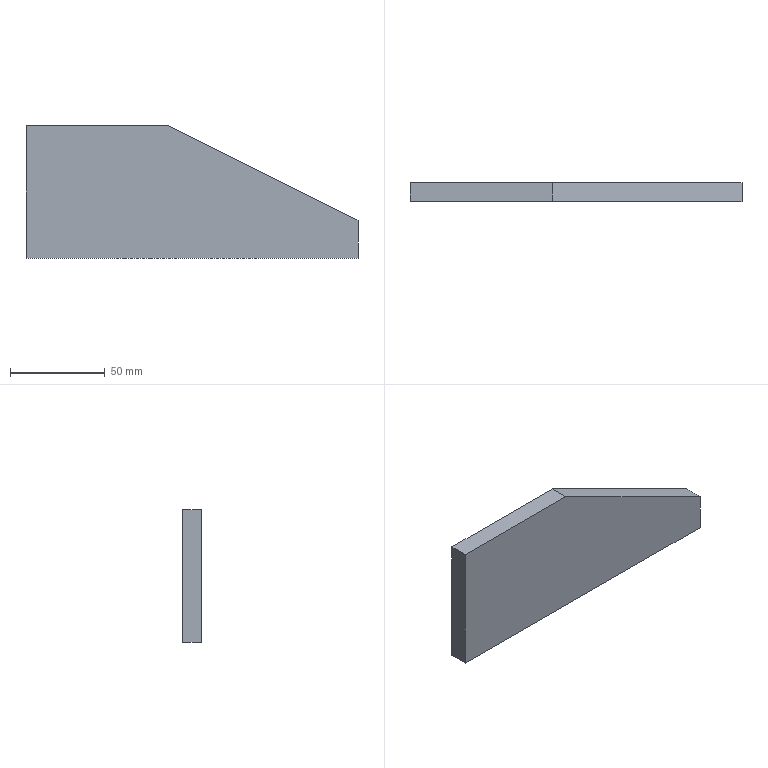Part | STEP file | Positioning_id2130_x_t | 1 solid | 7 faces | box 175 x 10 x 70 mm | volume 97500 mm3 | plane 7
STEP:
#1=CARTESIAN_POINT('',(0.,0.,0.));
#2=DIRECTION('',(0.,0.,1.));
#3=DIRECTION('',(1.,0.,0.));
#4=AXIS2_PLACEMENT_3D('',#1,#2,#3);
#5=CARTESIAN_POINT('',(-823.002,196.5,393.532));
#6=VERTEX_POINT('',#5);
#7=CARTESIAN_POINT('',(-923.002,196.5,443.532));
#8=VERTEX_POINT('',#7);
#9=CARTESIAN_POINT('',(-823.002,196.5,393.532));
#10=DIRECTION('',(-0.8944,0.,0.4472));
#11=VECTOR('',#10,1.);
#12=LINE('',#9,#11);
#13=CARTESIAN_POINT('',(-923.002,201.5,443.532));
#14=DIRECTION('',(-0.4472,0.,-0.8944));
#15=DIRECTION('',(0.8944,0.,-0.4472));
#16=AXIS2_PLACEMENT_3D('',#13,#14,#15);
#17=PLANE('',#16);
#18=CARTESIAN_POINT('',(111.803,5.));
#19=DIRECTION('',(-1.,0.));
#20=VECTOR('',#19,1.);
#21=LINE('',#18,#20);
#22=(GEOMETRIC_REPRESENTATION_CONTEXT(2)PARAMETRIC_REPRESENTATION_CONTEXT()REPRESENTATION_CONTEXT('',''));
#23=DEFINITIONAL_REPRESENTATION('',(#21),#22);
#24=PCURVE('',#17,#23);
#25=CARTESIAN_POINT('',(-893.002,196.5,413.532));
#26=DIRECTION('',(0.,-1.,0.));
#27=DIRECTION('',(1.,0.,0.));
#28=AXIS2_PLACEMENT_3D('',#25,#26,#27);
#29=PLANE('',#28);
#30=CARTESIAN_POINT('',(70.,-20.));
#31=DIRECTION('',(-0.8944,0.4472));
#32=VECTOR('',#31,1.);
#33=LINE('',#30,#32);
#34=(GEOMETRIC_REPRESENTATION_CONTEXT(2)PARAMETRIC_REPRESENTATION_CONTEXT()REPRESENTATION_CONTEXT('',''));
#35=DEFINITIONAL_REPRESENTATION('',(#33),#34);
#36=PCURVE('',#29,#35);
#37=SURFACE_CURVE('',#12,(#24,#36),.PCURVE_S1.);
#38=EDGE_CURVE('',#6,#8,#37,.T.);
#39=ORIENTED_EDGE('',*,*,#38,.F.);
#40=CARTESIAN_POINT('',(-823.002,206.5,393.532));
#41=VERTEX_POINT('',#40);
#42=CARTESIAN_POINT('',(-823.002,206.5,393.532));
#43=DIRECTION('',(0.,-1.,0.));
#44=VECTOR('',#43,1.);
#45=LINE('',#42,#44);
#46=CARTESIAN_POINT('',(111.803,-5.));
#47=DIRECTION('',(0.,1.));
#48=VECTOR('',#47,1.);
#49=LINE('',#46,#48);
#50=(GEOMETRIC_REPRESENTATION_CONTEXT(2)PARAMETRIC_REPRESENTATION_CONTEXT()REPRESENTATION_CONTEXT('',''));
#51=DEFINITIONAL_REPRESENTATION('',(#49),#50);
#52=PCURVE('',#17,#51);
#53=CARTESIAN_POINT('',(-823.002,201.5,413.532));
#54=DIRECTION('',(1.,0.,0.));
#55=DIRECTION('',(0.,1.,0.));
#56=AXIS2_PLACEMENT_3D('',#53,#54,#55);
#57=PLANE('',#56);
#58=CARTESIAN_POINT('',(5.,-20.));
#59=DIRECTION('',(-1.,0.));
#60=VECTOR('',#59,1.);
#61=LINE('',#58,#60);
#62=(GEOMETRIC_REPRESENTATION_CONTEXT(2)PARAMETRIC_REPRESENTATION_CONTEXT()REPRESENTATION_CONTEXT('',''));
#63=DEFINITIONAL_REPRESENTATION('',(#61),#62);
#64=PCURVE('',#57,#63);
#65=SURFACE_CURVE('',#45,(#52,#64),.PCURVE_S1.);
#66=EDGE_CURVE('',#41,#6,#65,.T.);
#67=ORIENTED_EDGE('',*,*,#66,.F.);
#68=CARTESIAN_POINT('',(-923.002,206.5,443.532));
#69=VERTEX_POINT('',#68);
#70=CARTESIAN_POINT('',(-923.002,206.5,443.532));
#71=DIRECTION('',(0.8944,0.,-0.4472));
#72=VECTOR('',#71,1.);
#73=LINE('',#70,#72);
#74=CARTESIAN_POINT('',(0.,-5.));
#75=DIRECTION('',(1.,0.));
#76=VECTOR('',#75,1.);
#77=LINE('',#74,#76);
#78=(GEOMETRIC_REPRESENTATION_CONTEXT(2)PARAMETRIC_REPRESENTATION_CONTEXT()REPRESENTATION_CONTEXT('',''));
#79=DEFINITIONAL_REPRESENTATION('',(#77),#78);
#80=PCURVE('',#17,#79);
#81=CARTESIAN_POINT('',(-893.002,206.5,413.532));
#82=DIRECTION('',(0.,1.,0.));
#83=DIRECTION('',(-1.,0.,0.));
#84=AXIS2_PLACEMENT_3D('',#81,#82,#83);
#85=PLANE('',#84);
#86=CARTESIAN_POINT('',(30.,30.));
#87=DIRECTION('',(-0.8944,-0.4472));
#88=VECTOR('',#87,1.);
#89=LINE('',#86,#88);
#90=(GEOMETRIC_REPRESENTATION_CONTEXT(2)PARAMETRIC_REPRESENTATION_CONTEXT()REPRESENTATION_CONTEXT('',''));
#91=DEFINITIONAL_REPRESENTATION('',(#89),#90);
#92=PCURVE('',#85,#91);
#93=SURFACE_CURVE('',#73,(#80,#92),.PCURVE_S1.);
#94=EDGE_CURVE('',#69,#41,#93,.T.);
#95=ORIENTED_EDGE('',*,*,#94,.F.);
#96=CARTESIAN_POINT('',(-923.002,196.5,443.532));
#97=DIRECTION('',(0.,1.,0.));
#98=VECTOR('',#97,1.);
#99=LINE('',#96,#98);
#100=CARTESIAN_POINT('',(0.,5.));
#101=DIRECTION('',(0.,-1.));
#102=VECTOR('',#101,1.);
#103=LINE('',#100,#102);
#104=(GEOMETRIC_REPRESENTATION_CONTEXT(2)PARAMETRIC_REPRESENTATION_CONTEXT()REPRESENTATION_CONTEXT('',''));
#105=DEFINITIONAL_REPRESENTATION('',(#103),#104);
#106=PCURVE('',#17,#105);
#107=CARTESIAN_POINT('',(-893.002,201.5,443.532));
#108=DIRECTION('',(0.,0.,1.));
#109=DIRECTION('',(0.,-1.,0.));
#110=AXIS2_PLACEMENT_3D('',#107,#108,#109);
#111=PLANE('',#110);
#112=CARTESIAN_POINT('',(5.,-30.));
#113=DIRECTION('',(-1.,0.));
#114=VECTOR('',#113,1.);
#115=LINE('',#112,#114);
#116=(GEOMETRIC_REPRESENTATION_CONTEXT(2)PARAMETRIC_REPRESENTATION_CONTEXT()REPRESENTATION_CONTEXT('',''));
#117=DEFINITIONAL_REPRESENTATION('',(#115),#116);
#118=PCURVE('',#111,#117);
#119=SURFACE_CURVE('',#99,(#106,#118),.PCURVE_S1.);
#120=EDGE_CURVE('',#8,#69,#119,.T.);
#121=ORIENTED_EDGE('',*,*,#120,.F.);
#122=EDGE_LOOP('',(#39,#67,#95,#121));
#123=FACE_BOUND('',#122,.T.);
#124=ADVANCED_FACE('',(#123),#17,.F.);
#125=CARTESIAN_POINT('',(-823.002,206.5,373.532));
#126=VERTEX_POINT('',#125);
#127=CARTESIAN_POINT('',(-823.002,206.5,393.532));
#128=DIRECTION('',(0.,0.,-1.));
#129=VECTOR('',#128,1.);
#130=LINE('',#127,#129);
#131=CARTESIAN_POINT('',(5.,-20.));
#132=DIRECTION('',(0.,-1.));
#133=VECTOR('',#132,1.);
#134=LINE('',#131,#133);
#135=(GEOMETRIC_REPRESENTATION_CONTEXT(2)PARAMETRIC_REPRESENTATION_CONTEXT()REPRESENTATION_CONTEXT('',''));
#136=DEFINITIONAL_REPRESENTATION('',(#134),#135);
#137=PCURVE('',#57,#136);
#138=CARTESIAN_POINT('',(-70.,-20.));
#139=DIRECTION('',(0.,-1.));
#140=VECTOR('',#139,1.);
#141=LINE('',#138,#140);
#142=(GEOMETRIC_REPRESENTATION_CONTEXT(2)PARAMETRIC_REPRESENTATION_CONTEXT()REPRESENTATION_CONTEXT('',''));
#143=DEFINITIONAL_REPRESENTATION('',(#141),#142);
#144=PCURVE('',#85,#143);
#145=SURFACE_CURVE('',#130,(#137,#144),.PCURVE_S1.);
#146=EDGE_CURVE('',#41,#126,#145,.T.);
#147=ORIENTED_EDGE('',*,*,#146,.F.);
#148=ORIENTED_EDGE('',*,*,#66,.T.);
#149=CARTESIAN_POINT('',(-823.002,196.5,373.532));
#150=VERTEX_POINT('',#149);
#151=CARTESIAN_POINT('',(-823.002,196.5,373.532));
#152=DIRECTION('',(0.,0.,1.));
#153=VECTOR('',#152,1.);
#154=LINE('',#151,#153);
#155=CARTESIAN_POINT('',(-5.,-40.));
#156=DIRECTION('',(0.,1.));
#157=VECTOR('',#156,1.);
#158=LINE('',#155,#157);
#159=(GEOMETRIC_REPRESENTATION_CONTEXT(2)PARAMETRIC_REPRESENTATION_CONTEXT()REPRESENTATION_CONTEXT('',''));
#160=DEFINITIONAL_REPRESENTATION('',(#158),#159);
#161=PCURVE('',#57,#160);
#162=CARTESIAN_POINT('',(70.,-40.));
#163=DIRECTION('',(0.,1.));
#164=VECTOR('',#163,1.);
#165=LINE('',#162,#164);
#166=(GEOMETRIC_REPRESENTATION_CONTEXT(2)PARAMETRIC_REPRESENTATION_CONTEXT()REPRESENTATION_CONTEXT('',''));
#167=DEFINITIONAL_REPRESENTATION('',(#165),#166);
#168=PCURVE('',#29,#167);
#169=SURFACE_CURVE('',#154,(#161,#168),.PCURVE_S1.);
#170=EDGE_CURVE('',#150,#6,#169,.T.);
#171=ORIENTED_EDGE('',*,*,#170,.F.);
#172=CARTESIAN_POINT('',(-823.002,196.5,373.532));
#173=DIRECTION('',(0.,1.,0.));
#174=VECTOR('',#173,1.);
#175=LINE('',#172,#174);
#176=CARTESIAN_POINT('',(-5.,-40.));
#177=DIRECTION('',(1.,0.));
#178=VECTOR('',#177,1.);
#179=LINE('',#176,#178);
#180=(GEOMETRIC_REPRESENTATION_CONTEXT(2)PARAMETRIC_REPRESENTATION_CONTEXT()REPRESENTATION_CONTEXT('',''));
#181=DEFINITIONAL_REPRESENTATION('',(#179),#180);
#182=PCURVE('',#57,#181);
#183=CARTESIAN_POINT('',(-893.002,201.5,373.532));
#184=DIRECTION('',(0.,0.,-1.));
#185=DIRECTION('',(0.,1.,0.));
#186=AXIS2_PLACEMENT_3D('',#183,#184,#185);
#187=PLANE('',#186);
#188=CARTESIAN_POINT('',(-5.,70.));
#189=DIRECTION('',(1.,0.));
#190=VECTOR('',#189,1.);
#191=LINE('',#188,#190);
#192=(GEOMETRIC_REPRESENTATION_CONTEXT(2)PARAMETRIC_REPRESENTATION_CONTEXT()REPRESENTATION_CONTEXT('',''));
#193=DEFINITIONAL_REPRESENTATION('',(#191),#192);
#194=PCURVE('',#187,#193);
#195=SURFACE_CURVE('',#175,(#182,#194),.PCURVE_S1.);
#196=EDGE_CURVE('',#150,#126,#195,.T.);
#197=ORIENTED_EDGE('',*,*,#196,.T.);
#198=EDGE_LOOP('',(#147,#148,#171,#197));
#199=FACE_BOUND('',#198,.T.);
#200=ADVANCED_FACE('',(#199),#57,.T.);
#201=ORIENTED_EDGE('',*,*,#170,.T.);
#202=ORIENTED_EDGE('',*,*,#38,.T.);
#203=CARTESIAN_POINT('',(-998.002,196.5,443.532));
#204=VERTEX_POINT('',#203);
#205=CARTESIAN_POINT('',(-923.002,196.5,443.532));
#206=DIRECTION('',(-1.,0.,0.));
#207=VECTOR('',#206,1.);
#208=LINE('',#205,#207);
#209=CARTESIAN_POINT('',(-30.,30.));
#210=DIRECTION('',(-1.,0.));
#211=VECTOR('',#210,1.);
#212=LINE('',#209,#211);
#213=(GEOMETRIC_REPRESENTATION_CONTEXT(2)PARAMETRIC_REPRESENTATION_CONTEXT()REPRESENTATION_CONTEXT('',''));
#214=DEFINITIONAL_REPRESENTATION('',(#212),#213);
#215=PCURVE('',#29,#214);
#216=CARTESIAN_POINT('',(5.,-30.));
#217=DIRECTION('',(0.,-1.));
#218=VECTOR('',#217,1.);
#219=LINE('',#216,#218);
#220=(GEOMETRIC_REPRESENTATION_CONTEXT(2)PARAMETRIC_REPRESENTATION_CONTEXT()REPRESENTATION_CONTEXT('',''));
#221=DEFINITIONAL_REPRESENTATION('',(#219),#220);
#222=PCURVE('',#111,#221);
#223=SURFACE_CURVE('',#208,(#215,#222),.PCURVE_S1.);
#224=EDGE_CURVE('',#8,#204,#223,.T.);
#225=ORIENTED_EDGE('',*,*,#224,.T.);
#226=CARTESIAN_POINT('',(-998.002,196.5,373.532));
#227=VERTEX_POINT('',#226);
#228=CARTESIAN_POINT('',(-998.002,196.5,443.532));
#229=DIRECTION('',(0.,0.,-1.));
#230=VECTOR('',#229,1.);
#231=LINE('',#228,#230);
#232=CARTESIAN_POINT('',(-105.,30.));
#233=DIRECTION('',(0.,-1.));
#234=VECTOR('',#233,1.);
#235=LINE('',#232,#234);
#236=(GEOMETRIC_REPRESENTATION_CONTEXT(2)PARAMETRIC_REPRESENTATION_CONTEXT()REPRESENTATION_CONTEXT('',''));
#237=DEFINITIONAL_REPRESENTATION('',(#235),#236);
#238=PCURVE('',#29,#237);
#239=CARTESIAN_POINT('',(-998.002,201.5,413.532));
#240=DIRECTION('',(-1.,0.,0.));
#241=DIRECTION('',(0.,-1.,0.));
#242=AXIS2_PLACEMENT_3D('',#239,#240,#241);
#243=PLANE('',#242);
#244=CARTESIAN_POINT('',(5.,30.));
#245=DIRECTION('',(0.,-1.));
#246=VECTOR('',#245,1.);
#247=LINE('',#244,#246);
#248=(GEOMETRIC_REPRESENTATION_CONTEXT(2)PARAMETRIC_REPRESENTATION_CONTEXT()REPRESENTATION_CONTEXT('',''));
#249=DEFINITIONAL_REPRESENTATION('',(#247),#248);
#250=PCURVE('',#243,#249);
#251=SURFACE_CURVE('',#231,(#238,#250),.PCURVE_S1.);
#252=EDGE_CURVE('',#204,#227,#251,.T.);
#253=ORIENTED_EDGE('',*,*,#252,.T.);
#254=CARTESIAN_POINT('',(-998.002,196.5,373.532));
#255=DIRECTION('',(1.,0.,0.));
#256=VECTOR('',#255,1.);
#257=LINE('',#254,#256);
#258=CARTESIAN_POINT('',(-105.,-40.));
#259=DIRECTION('',(1.,0.));
#260=VECTOR('',#259,1.);
#261=LINE('',#258,#260);
#262=(GEOMETRIC_REPRESENTATION_CONTEXT(2)PARAMETRIC_REPRESENTATION_CONTEXT()REPRESENTATION_CONTEXT('',''));
#263=DEFINITIONAL_REPRESENTATION('',(#261),#262);
#264=PCURVE('',#29,#263);
#265=CARTESIAN_POINT('',(-5.,-105.));
#266=DIRECTION('',(0.,1.));
#267=VECTOR('',#266,1.);
#268=LINE('',#265,#267);
#269=(GEOMETRIC_REPRESENTATION_CONTEXT(2)PARAMETRIC_REPRESENTATION_CONTEXT()REPRESENTATION_CONTEXT('',''));
#270=DEFINITIONAL_REPRESENTATION('',(#268),#269);
#271=PCURVE('',#187,#270);
#272=SURFACE_CURVE('',#257,(#264,#271),.PCURVE_S1.);
#273=EDGE_CURVE('',#227,#150,#272,.T.);
#274=ORIENTED_EDGE('',*,*,#273,.T.);
#275=EDGE_LOOP('',(#201,#202,#225,#253,#274));
#276=FACE_BOUND('',#275,.T.);
#277=ADVANCED_FACE('',(#276),#29,.T.);
#278=ORIENTED_EDGE('',*,*,#224,.F.);
#279=ORIENTED_EDGE('',*,*,#120,.T.);
#280=CARTESIAN_POINT('',(-998.002,206.5,443.532));
#281=VERTEX_POINT('',#280);
#282=CARTESIAN_POINT('',(-998.002,206.5,443.532));
#283=DIRECTION('',(1.,0.,0.));
#284=VECTOR('',#283,1.);
#285=LINE('',#282,#284);
#286=CARTESIAN_POINT('',(-5.,-105.));
#287=DIRECTION('',(0.,1.));
#288=VECTOR('',#287,1.);
#289=LINE('',#286,#288);
#290=(GEOMETRIC_REPRESENTATION_CONTEXT(2)PARAMETRIC_REPRESENTATION_CONTEXT()REPRESENTATION_CONTEXT('',''));
#291=DEFINITIONAL_REPRESENTATION('',(#289),#290);
#292=PCURVE('',#111,#291);
#293=CARTESIAN_POINT('',(105.,30.));
#294=DIRECTION('',(-1.,0.));
#295=VECTOR('',#294,1.);
#296=LINE('',#293,#295);
#297=(GEOMETRIC_REPRESENTATION_CONTEXT(2)PARAMETRIC_REPRESENTATION_CONTEXT()REPRESENTATION_CONTEXT('',''));
#298=DEFINITIONAL_REPRESENTATION('',(#296),#297);
#299=PCURVE('',#85,#298);
#300=SURFACE_CURVE('',#285,(#292,#299),.PCURVE_S1.);
#301=EDGE_CURVE('',#281,#69,#300,.T.);
#302=ORIENTED_EDGE('',*,*,#301,.F.);
#303=CARTESIAN_POINT('',(-998.002,196.5,443.532));
#304=DIRECTION('',(0.,1.,0.));
#305=VECTOR('',#304,1.);
#306=LINE('',#303,#305);
#307=CARTESIAN_POINT('',(5.,-105.));
#308=DIRECTION('',(-1.,0.));
#309=VECTOR('',#308,1.);
#310=LINE('',#307,#309);
#311=(GEOMETRIC_REPRESENTATION_CONTEXT(2)PARAMETRIC_REPRESENTATION_CONTEXT()REPRESENTATION_CONTEXT('',''));
#312=DEFINITIONAL_REPRESENTATION('',(#310),#311);
#313=PCURVE('',#111,#312);
#314=CARTESIAN_POINT('',(5.,30.));
#315=DIRECTION('',(-1.,0.));
#316=VECTOR('',#315,1.);
#317=LINE('',#314,#316);
#318=(GEOMETRIC_REPRESENTATION_CONTEXT(2)PARAMETRIC_REPRESENTATION_CONTEXT()REPRESENTATION_CONTEXT('',''));
#319=DEFINITIONAL_REPRESENTATION('',(#317),#318);
#320=PCURVE('',#243,#319);
#321=SURFACE_CURVE('',#306,(#313,#320),.PCURVE_S1.);
#322=EDGE_CURVE('',#204,#281,#321,.T.);
#323=ORIENTED_EDGE('',*,*,#322,.F.);
#324=EDGE_LOOP('',(#278,#279,#302,#323));
#325=FACE_BOUND('',#324,.T.);
#326=ADVANCED_FACE('',(#325),#111,.T.);
#327=CARTESIAN_POINT('',(-998.002,206.5,373.532));
#328=VERTEX_POINT('',#327);
#329=CARTESIAN_POINT('',(-998.002,196.5,373.532));
#330=DIRECTION('',(0.,1.,0.));
#331=VECTOR('',#330,1.);
#332=LINE('',#329,#331);
#333=CARTESIAN_POINT('',(5.,-40.));
#334=DIRECTION('',(-1.,0.));
#335=VECTOR('',#334,1.);
#336=LINE('',#333,#335);
#337=(GEOMETRIC_REPRESENTATION_CONTEXT(2)PARAMETRIC_REPRESENTATION_CONTEXT()REPRESENTATION_CONTEXT('',''));
#338=DEFINITIONAL_REPRESENTATION('',(#336),#337);
#339=PCURVE('',#243,#338);
#340=CARTESIAN_POINT('',(-5.,-105.));
#341=DIRECTION('',(1.,0.));
#342=VECTOR('',#341,1.);
#343=LINE('',#340,#342);
#344=(GEOMETRIC_REPRESENTATION_CONTEXT(2)PARAMETRIC_REPRESENTATION_CONTEXT()REPRESENTATION_CONTEXT('',''));
#345=DEFINITIONAL_REPRESENTATION('',(#343),#344);
#346=PCURVE('',#187,#345);
#347=SURFACE_CURVE('',#332,(#339,#346),.PCURVE_S1.);
#348=EDGE_CURVE('',#227,#328,#347,.T.);
#349=ORIENTED_EDGE('',*,*,#348,.F.);
#350=ORIENTED_EDGE('',*,*,#252,.F.);
#351=ORIENTED_EDGE('',*,*,#322,.T.);
#352=CARTESIAN_POINT('',(-998.002,206.5,373.532));
#353=DIRECTION('',(0.,0.,1.));
#354=VECTOR('',#353,1.);
#355=LINE('',#352,#354);
#356=CARTESIAN_POINT('',(-5.,-40.));
#357=DIRECTION('',(0.,1.));
#358=VECTOR('',#357,1.);
#359=LINE('',#356,#358);
#360=(GEOMETRIC_REPRESENTATION_CONTEXT(2)PARAMETRIC_REPRESENTATION_CONTEXT()REPRESENTATION_CONTEXT('',''));
#361=DEFINITIONAL_REPRESENTATION('',(#359),#360);
#362=PCURVE('',#243,#361);
#363=CARTESIAN_POINT('',(105.,-40.));
#364=DIRECTION('',(0.,1.));
#365=VECTOR('',#364,1.);
#366=LINE('',#363,#365);
#367=(GEOMETRIC_REPRESENTATION_CONTEXT(2)PARAMETRIC_REPRESENTATION_CONTEXT()REPRESENTATION_CONTEXT('',''));
#368=DEFINITIONAL_REPRESENTATION('',(#366),#367);
#369=PCURVE('',#85,#368);
#370=SURFACE_CURVE('',#355,(#362,#369),.PCURVE_S1.);
#371=EDGE_CURVE('',#328,#281,#370,.T.);
#372=ORIENTED_EDGE('',*,*,#371,.F.);
#373=EDGE_LOOP('',(#349,#350,#351,#372));
#374=FACE_BOUND('',#373,.T.);
#375=ADVANCED_FACE('',(#374),#243,.T.);
#376=ORIENTED_EDGE('',*,*,#196,.F.);
#377=ORIENTED_EDGE('',*,*,#273,.F.);
#378=ORIENTED_EDGE('',*,*,#348,.T.);
#379=CARTESIAN_POINT('',(-823.002,206.5,373.532));
#380=DIRECTION('',(-1.,0.,0.));
#381=VECTOR('',#380,1.);
#382=LINE('',#379,#381);
#383=CARTESIAN_POINT('',(5.,70.));
#384=DIRECTION('',(0.,-1.));
#385=VECTOR('',#384,1.);
#386=LINE('',#383,#385);
#387=(GEOMETRIC_REPRESENTATION_CONTEXT(2)PARAMETRIC_REPRESENTATION_CONTEXT()REPRESENTATION_CONTEXT('',''));
#388=DEFINITIONAL_REPRESENTATION('',(#386),#387);
#389=PCURVE('',#187,#388);
#390=CARTESIAN_POINT('',(-70.,-40.));
#391=DIRECTION('',(1.,0.));
#392=VECTOR('',#391,1.);
#393=LINE('',#390,#392);
#394=(GEOMETRIC_REPRESENTATION_CONTEXT(2)PARAMETRIC_REPRESENTATION_CONTEXT()REPRESENTATION_CONTEXT('',''));
#395=DEFINITIONAL_REPRESENTATION('',(#393),#394);
#396=PCURVE('',#85,#395);
#397=SURFACE_CURVE('',#382,(#389,#396),.PCURVE_S1.);
#398=EDGE_CURVE('',#126,#328,#397,.T.);
#399=ORIENTED_EDGE('',*,*,#398,.F.);
#400=EDGE_LOOP('',(#376,#377,#378,#399));
#401=FACE_BOUND('',#400,.T.);
#402=ADVANCED_FACE('',(#401),#187,.T.);
#403=ORIENTED_EDGE('',*,*,#301,.T.);
#404=ORIENTED_EDGE('',*,*,#94,.T.);
#405=ORIENTED_EDGE('',*,*,#146,.T.);
#406=ORIENTED_EDGE('',*,*,#398,.T.);
#407=ORIENTED_EDGE('',*,*,#371,.T.);
#408=EDGE_LOOP('',(#403,#404,#405,#406,#407));
#409=FACE_BOUND('',#408,.T.);
#410=ADVANCED_FACE('',(#409),#85,.T.);
#411=CLOSED_SHELL('',(#124,#200,#277,#326,#375,#402,#410));
#412=MANIFOLD_SOLID_BREP('',#411);
#413=(LENGTH_UNIT()NAMED_UNIT(*)SI_UNIT(.MILLI.,.METRE.));
#414=UNCERTAINTY_MEASURE_WITH_UNIT(LENGTH_MEASURE(0.0000001),#413,'','');
#415=(NAMED_UNIT(*)PLANE_ANGLE_UNIT()SI_UNIT($,.RADIAN.));
#416=(NAMED_UNIT(*)SI_UNIT($,.STERADIAN.)SOLID_ANGLE_UNIT());
#417=(GEOMETRIC_REPRESENTATION_CONTEXT(3)GLOBAL_UNCERTAINTY_ASSIGNED_CONTEXT((#414))GLOBAL_UNIT_ASSIGNED_CONTEXT((#413,#415,#416))REPRESENTATION_CONTEXT('',''));
#418=ADVANCED_BREP_SHAPE_REPRESENTATION('',(#4,#412),#417);